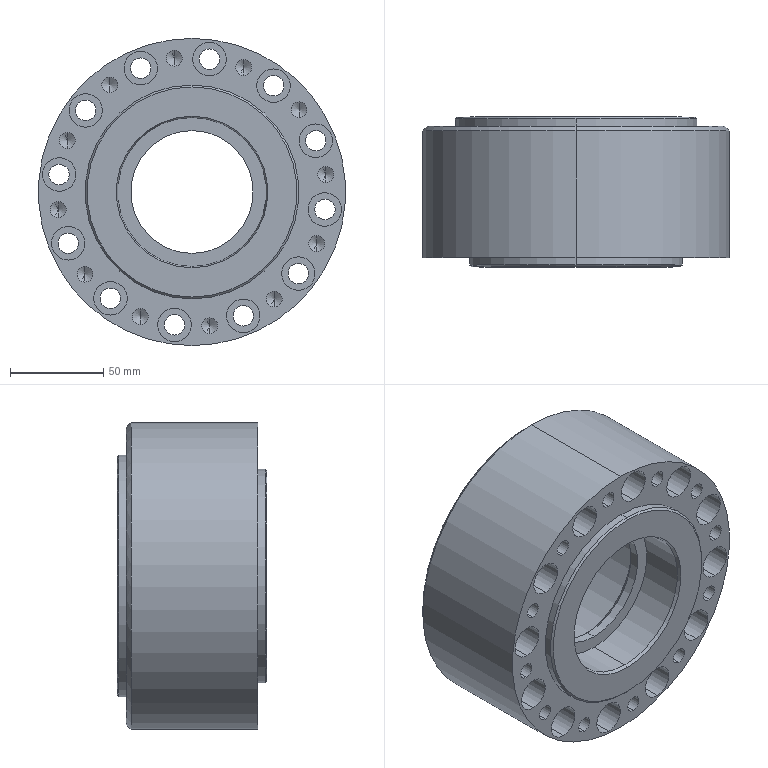Part | SolidWorks | features ICE 9, Chamfer 7, HoleWzd 5, CirPattern 3, Extrusion 1, RefAxis 1 | 1 solid | 157 faces | box 165 x 80.5 x 165 mm | volume 868351 mm3 | cylinder 92 | cone 46 | plane 19 | commonest cylinder face diameters 8.5 x24 11 x24 18 x24 3.3 x8 66 x2 80 x2